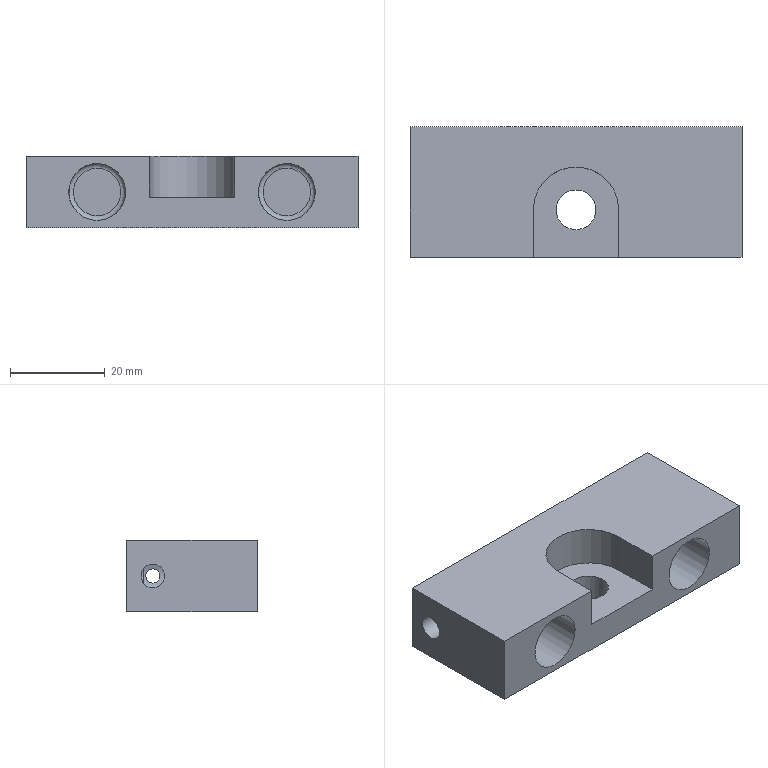NC program | NX | posted with a generic post | part box 70 x 27.5 x 15 mm
Whole program:
N10 G17 G21 G94 G90
(DRILLING , TOOL : 点孔D10-90-90度)
N12 T07 M6
N14 G54
N16 G17 G0 G90 X22. Y-7.5 B0. C0. S1600 M3
N18 G43 Z20. H7
N20 G94 G81 G99 Z-1.5 B-180. C-90. F150. R3.
N22 G80
N24 G0 X22. Y-7.5 Z20.
N26 M5
(DRILLING_1_COPY , TOOL : 钻头D5.1-62-92)
N28 T08 M6
N30 G54
N32 G17 G0 G90 X22. Y-7.5 B0. C0. S1800 M3
N34 G43 Z20. H8
N36 G94 G83 G99 Z-15. B-180. C-90. F150. Q2. R3.
N38 G80
N40 G0 X22. Y-7.5 Z20.
N42 M5
(DRILLING_1 , TOOL : 钻头D3.0-42-71)
N44 T09 M6
N46 G54
N48 G17 G0 G90 X22. Y-7.5 B0. C0. S1600 M3
N50 G43 Z20. H9
N52 G94 G83 G99 Z-51. B-180. C-90. F80. Q2. R3.
N54 G80
N56 G0 X22. Y-7.5 Z20.
N58 M5
(DRILLING_1_COPY_COPY , TOOL : 上排M6-23-D6-63)
N60 T10 M6
N62 G54
N64 G17 G0 G90 X22. Y-7.5 B0. C0. S300 M3
N66 G43 Z20. H10
N68 G84 G94 G99 Z-5. B-180. C-90. F300. R3.
N70 G80
N72 G0 X22. Y-7.5 Z20.
N74 M5
N76 M2